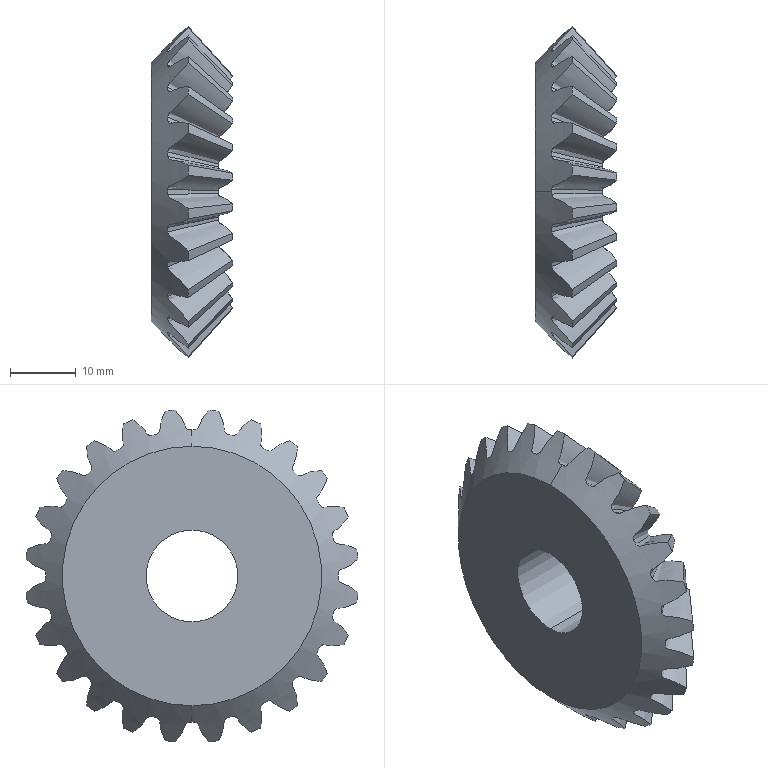Part | SolidWorks | features 3DProfileFeature 12, BlendCut 1, CirPattern 1, ICE 1, RefAxis 1, Revolution 1 | 1 solid | 104 faces | box 12.427 x 50.574 x 50.574 mm | volume 13201 mm3 | spline 48 | cone 28 | plane 26 | cylinder 2 | commonest cylinder face diameters 14 x2